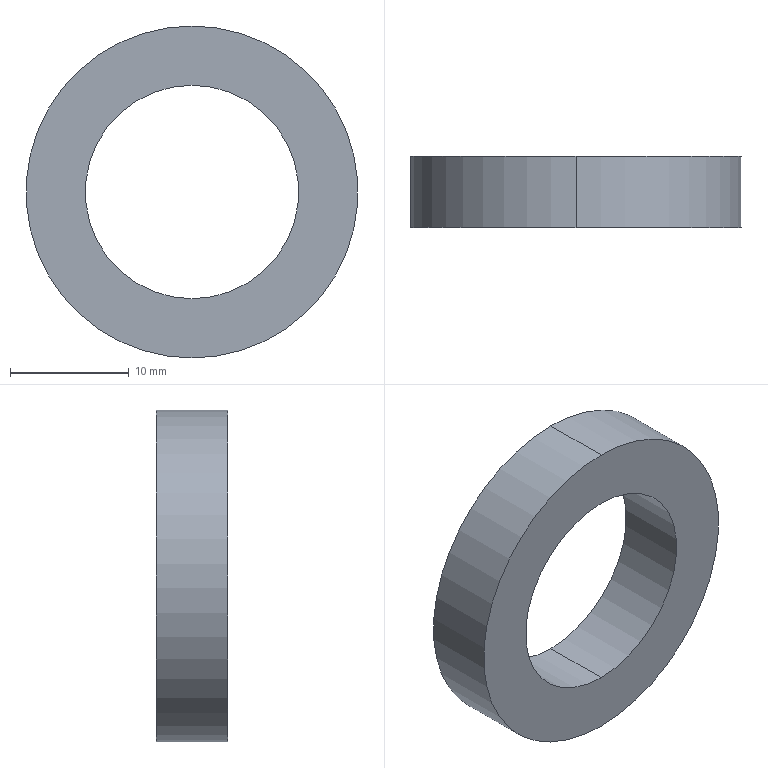Part | SolidWorks | features FlatPattern 1, SMBaseFlange 1, SheetMetal 1 | 1 solid | 6 faces | box 28 x 6 x 28 mm | volume 2168 mm3 | cylinder 4 | plane 2 | commonest cylinder face diameters 18 x2 28 x2
STEP:
#1=CARTESIAN_POINT('',(0.,-6.,-9.));
#2=VERTEX_POINT('',#1);
#3=CARTESIAN_POINT('',(0.,-6.,9.));
#4=VERTEX_POINT('',#3);
#5=CARTESIAN_POINT('',(0.,-6.,0.));
#6=DIRECTION('',(0.,1.,0.));
#7=DIRECTION('',(0.,0.,1.));
#8=AXIS2_PLACEMENT_3D('',#5,#6,#7);
#9=CIRCLE('',#8,9.);
#10=EDGE_CURVE('',#2,#4,#9,.T.);
#11=ORIENTED_EDGE('',*,*,#10,.F.);
#12=CARTESIAN_POINT('',(0.,0.,-9.));
#13=VERTEX_POINT('',#12);
#14=CARTESIAN_POINT('',(0.,-6.,-9.));
#15=DIRECTION('',(0.,1.,0.));
#16=VECTOR('',#15,1000.);
#17=LINE('',#14,#16);
#18=EDGE_CURVE('',#2,#13,#17,.T.);
#19=ORIENTED_EDGE('',*,*,#18,.T.);
#20=CARTESIAN_POINT('',(0.,0.,9.));
#21=VERTEX_POINT('',#20);
#22=CARTESIAN_POINT('',(0.,0.,0.));
#23=DIRECTION('',(0.,1.,0.));
#24=DIRECTION('',(0.,0.,1.));
#25=AXIS2_PLACEMENT_3D('',#22,#23,#24);
#26=CIRCLE('',#25,9.);
#27=EDGE_CURVE('',#13,#21,#26,.T.);
#28=ORIENTED_EDGE('',*,*,#27,.T.);
#29=CARTESIAN_POINT('',(0.,-6.,9.));
#30=DIRECTION('',(0.,1.,0.));
#31=VECTOR('',#30,1000.);
#32=LINE('',#29,#31);
#33=EDGE_CURVE('',#4,#21,#32,.T.);
#34=ORIENTED_EDGE('',*,*,#33,.F.);
#35=EDGE_LOOP('',(#11,#19,#28,#34));
#36=FACE_OUTER_BOUND('',#35,.T.);
#37=CARTESIAN_POINT('',(0.,-6.,0.));
#38=DIRECTION('',(0.,1.,0.));
#39=DIRECTION('',(0.,0.,1.));
#40=AXIS2_PLACEMENT_3D('',#37,#38,#39);
#41=CYLINDRICAL_SURFACE('',#40,9.);
#42=ADVANCED_FACE('',(#36),#41,.F.);
#43=CARTESIAN_POINT('',(0.,-6.,14.));
#44=VERTEX_POINT('',#43);
#45=CARTESIAN_POINT('',(0.,-6.,-14.));
#46=VERTEX_POINT('',#45);
#47=CARTESIAN_POINT('',(0.,-6.,0.));
#48=DIRECTION('',(0.,1.,0.));
#49=DIRECTION('',(0.,0.,1.));
#50=AXIS2_PLACEMENT_3D('',#47,#48,#49);
#51=CIRCLE('',#50,14.);
#52=EDGE_CURVE('',#44,#46,#51,.T.);
#53=ORIENTED_EDGE('',*,*,#52,.T.);
#54=CARTESIAN_POINT('',(0.,0.,-14.));
#55=VERTEX_POINT('',#54);
#56=CARTESIAN_POINT('',(0.,-6.,-14.));
#57=DIRECTION('',(0.,1.,0.));
#58=VECTOR('',#57,1000.);
#59=LINE('',#56,#58);
#60=EDGE_CURVE('',#46,#55,#59,.T.);
#61=ORIENTED_EDGE('',*,*,#60,.T.);
#62=CARTESIAN_POINT('',(0.,0.,14.));
#63=VERTEX_POINT('',#62);
#64=CARTESIAN_POINT('',(0.,0.,0.));
#65=DIRECTION('',(0.,1.,0.));
#66=DIRECTION('',(0.,0.,1.));
#67=AXIS2_PLACEMENT_3D('',#64,#65,#66);
#68=CIRCLE('',#67,14.);
#69=EDGE_CURVE('',#63,#55,#68,.T.);
#70=ORIENTED_EDGE('',*,*,#69,.F.);
#71=CARTESIAN_POINT('',(0.,-6.,14.));
#72=DIRECTION('',(0.,1.,0.));
#73=VECTOR('',#72,1000.);
#74=LINE('',#71,#73);
#75=EDGE_CURVE('',#44,#63,#74,.T.);
#76=ORIENTED_EDGE('',*,*,#75,.F.);
#77=EDGE_LOOP('',(#53,#61,#70,#76));
#78=FACE_OUTER_BOUND('',#77,.T.);
#79=CARTESIAN_POINT('',(0.,-6.,0.));
#80=DIRECTION('',(0.,1.,0.));
#81=DIRECTION('',(0.,0.,1.));
#82=AXIS2_PLACEMENT_3D('',#79,#80,#81);
#83=CYLINDRICAL_SURFACE('',#82,14.);
#84=ADVANCED_FACE('',(#78),#83,.T.);
#85=ORIENTED_EDGE('',*,*,#60,.F.);
#86=CARTESIAN_POINT('',(0.,-6.,0.));
#87=DIRECTION('',(0.,1.,0.));
#88=DIRECTION('',(0.,0.,1.));
#89=AXIS2_PLACEMENT_3D('',#86,#87,#88);
#90=CIRCLE('',#89,14.);
#91=EDGE_CURVE('',#46,#44,#90,.T.);
#92=ORIENTED_EDGE('',*,*,#91,.T.);
#93=ORIENTED_EDGE('',*,*,#75,.T.);
#94=CARTESIAN_POINT('',(0.,0.,0.));
#95=DIRECTION('',(0.,1.,0.));
#96=DIRECTION('',(0.,0.,1.));
#97=AXIS2_PLACEMENT_3D('',#94,#95,#96);
#98=CIRCLE('',#97,14.);
#99=EDGE_CURVE('',#55,#63,#98,.T.);
#100=ORIENTED_EDGE('',*,*,#99,.F.);
#101=EDGE_LOOP('',(#85,#92,#93,#100));
#102=FACE_OUTER_BOUND('',#101,.T.);
#103=CARTESIAN_POINT('',(0.,-6.,0.));
#104=DIRECTION('',(0.,1.,0.));
#105=DIRECTION('',(0.,0.,1.));
#106=AXIS2_PLACEMENT_3D('',#103,#104,#105);
#107=CYLINDRICAL_SURFACE('',#106,14.);
#108=ADVANCED_FACE('',(#102),#107,.T.);
#109=CARTESIAN_POINT('',(0.,-6.,0.));
#110=DIRECTION('',(0.,1.,0.));
#111=DIRECTION('',(0.,0.,1.));
#112=AXIS2_PLACEMENT_3D('',#109,#110,#111);
#113=CIRCLE('',#112,9.);
#114=EDGE_CURVE('',#4,#2,#113,.T.);
#115=ORIENTED_EDGE('',*,*,#114,.T.);
#116=ORIENTED_EDGE('',*,*,#10,.T.);
#117=EDGE_LOOP('',(#115,#116));
#118=FACE_BOUND('',#117,.T.);
#119=ORIENTED_EDGE('',*,*,#52,.F.);
#120=ORIENTED_EDGE('',*,*,#91,.F.);
#121=EDGE_LOOP('',(#119,#120));
#122=FACE_OUTER_BOUND('',#121,.T.);
#123=CARTESIAN_POINT('',(0.,-6.,0.));
#124=DIRECTION('',(0.,1.,0.));
#125=DIRECTION('',(0.,0.,1.));
#126=AXIS2_PLACEMENT_3D('',#123,#124,#125);
#127=PLANE('',#126);
#128=ADVANCED_FACE('',(#118,#122),#127,.F.);
#129=CARTESIAN_POINT('',(0.,0.,0.));
#130=DIRECTION('',(0.,1.,0.));
#131=DIRECTION('',(0.,0.,1.));
#132=AXIS2_PLACEMENT_3D('',#129,#130,#131);
#133=CIRCLE('',#132,9.);
#134=EDGE_CURVE('',#21,#13,#133,.T.);
#135=ORIENTED_EDGE('',*,*,#134,.F.);
#136=ORIENTED_EDGE('',*,*,#27,.F.);
#137=EDGE_LOOP('',(#135,#136));
#138=FACE_BOUND('',#137,.T.);
#139=ORIENTED_EDGE('',*,*,#69,.T.);
#140=ORIENTED_EDGE('',*,*,#99,.T.);
#141=EDGE_LOOP('',(#139,#140));
#142=FACE_OUTER_BOUND('',#141,.T.);
#143=CARTESIAN_POINT('',(0.,0.,0.));
#144=DIRECTION('',(0.,1.,0.));
#145=DIRECTION('',(0.,0.,1.));
#146=AXIS2_PLACEMENT_3D('',#143,#144,#145);
#147=PLANE('',#146);
#148=ADVANCED_FACE('',(#138,#142),#147,.T.);
#149=ORIENTED_EDGE('',*,*,#18,.F.);
#150=ORIENTED_EDGE('',*,*,#114,.F.);
#151=ORIENTED_EDGE('',*,*,#33,.T.);
#152=ORIENTED_EDGE('',*,*,#134,.T.);
#153=EDGE_LOOP('',(#149,#150,#151,#152));
#154=FACE_OUTER_BOUND('',#153,.T.);
#155=CARTESIAN_POINT('',(0.,-6.,0.));
#156=DIRECTION('',(0.,1.,0.));
#157=DIRECTION('',(0.,0.,1.));
#158=AXIS2_PLACEMENT_3D('',#155,#156,#157);
#159=CYLINDRICAL_SURFACE('',#158,9.);
#160=ADVANCED_FACE('',(#154),#159,.F.);
#161=CLOSED_SHELL('',(#42,#84,#108,#128,#148,#160));
#162=MANIFOLD_SOLID_BREP('',#161);
#163=CARTESIAN_POINT('',(0.,0.,0.));
#164=DIRECTION('',(0.,0.,1.));
#165=DIRECTION('',(1.,0.,0.));
#166=AXIS2_PLACEMENT_3D('',#163,#164,#165);
#167=(LENGTH_UNIT()NAMED_UNIT(*)SI_UNIT(.MILLI.,.METRE.));
#168=UNCERTAINTY_MEASURE_WITH_UNIT(LENGTH_MEASURE(0.00001),#167,'','');
#169=(NAMED_UNIT(*)PLANE_ANGLE_UNIT()SI_UNIT($,.RADIAN.));
#170=(NAMED_UNIT(*)SI_UNIT($,.STERADIAN.)SOLID_ANGLE_UNIT());
#171=(GEOMETRIC_REPRESENTATION_CONTEXT(3)GLOBAL_UNCERTAINTY_ASSIGNED_CONTEXT((#168))GLOBAL_UNIT_ASSIGNED_CONTEXT((#167,#169,#170))REPRESENTATION_CONTEXT('',''));
#172=ADVANCED_BREP_SHAPE_REPRESENTATION('',(#162,#166),#171);